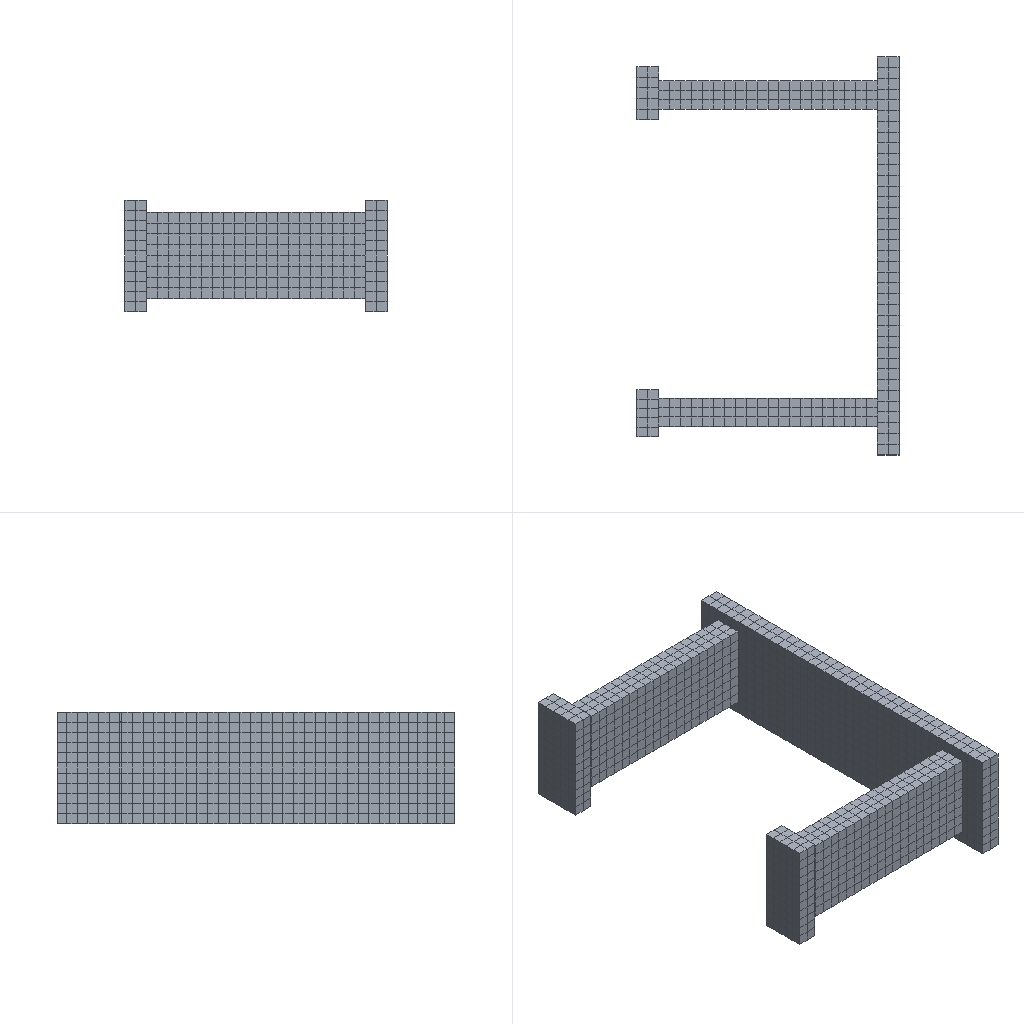Simulation study | ansys workbench
Set-up summary:
category,name,step,type,value,unit,region
solver,ansys_mapdl
solver,version,,,24.2
units,MPA,,stated
analysis,deck,,static,static
load_step,requested,,,1
analysis,nlgeom,,,False
mesh,nodes,,,11772
mesh,elements,,,2933
element_type,ANSYS 186 (type 1),,solid,110
element_type,ANSYS 186 (type 2),,solid,110
element_type,ANSYS 186 (type 3),,solid,480
element_type,ANSYS 186 (type 4),,solid,480
element_type,ANSYS 186 (type 5),,solid,814
element_type,ANSYS 174 (type 6),,contact,64
element_type,ANSYS 170 (type 7),,target,64
element_type,ANSYS 174 (type 8),,contact,74
element_type,ANSYS 170 (type 9),,target,74
element_type,ANSYS 174 (type 10),,contact,64
element_type,ANSYS 170 (type 11),,target,64
element_type,ANSYS 174 (type 12),,contact,64
element_type,ANSYS 170 (type 13),,target,64
element_type,ANSYS 154 (type 14),,surface,407
load,load commands in deck,,count,4
bc,support commands in deck,,count,1
named_set,_FIXEDSU,,component
material,1,,in results
material,2,,in results
material,3,,in results
material,4,,in results
material,5,,in results
check,setup vs results,,match,266 contact/target element(s) of the setup are not in the results: jiaoxue/qq_files/dp0/SYS/MECH/solve.out records that the solver deleted 266 by its trimming logic; 407 surface effect element(s) are not in the reader's mesh and were not compared
Ansys APDL input file, long lists of numbers shortened:
/batch
/config,noeldb,1     ! force off writing results to database
*get,_wallstrt,active,,time,wall
! ANSYS input file written by Workbench version 2024 R2
! File used for geometry attach: F:\jiaoxue\qq_files\dp0\SYS\DM\SYS.scdoc
/title,qq--____ (A5)
! ****** Begin Custom Load Command Snippet ******
/COM, ACT Extensions:
/COM,     LSDYNA, 2024.2
/COM,/COM,     ANSYSMotion, 2024.2
/COM,
! ****** End   Custom Load Command Snippet ******
*DIM,_wb_ProjectScratch_dir,string,248
_wb_ProjectScratch_dir(1) = 'F:\jiaoxue\_ProjectScratch\Scr3192\'
*DIM,_wb_SolverFiles_dir,string,248
_wb_SolverFiles_dir(1) = 'F:\jiaoxue\qq_files\dp0\SYS\MECH\'
*DIM,_wb_userfiles_dir,string,248
_wb_userfiles_dir(1) = 'F:\jiaoxue\qq_files\user_files\'
/com,--- Data in consistent NMM units. See Solving Units in the help system for more information.
/units,MPA
/nopr
/wb,file,start              !  signify a WB generated input file
/prep7
! Turn off shape checking because checks already performed inside WB mesher.
! See help system for more information.
SHPP,OFF,,NOWARN
/nolist
etcon,set             ! allow ANSYS to choose best KEYOP's for 180x elements, resets any applicable keyopt to MAPDL defaults
/com,*********** Nodes for the whole assembly ***********
nblock,3,,12949
(1i9,3e20.9e3)
        1    -1.050000000E+02     1.581539813E+02    -4.636363636E+01
! (11771 more lines like these left out)
-1
/wb,elem,start            !  set before creation of elements
/com,*********** Elements for Body 1 '1-prt0\__1' ***********
et,1,186
keyo,1,2,1          ! set full integration on SOLID186
eblock,19,solid,,110
(19i9)
        1        1        1        1        0        0        0        0       20        0        1        1      165      173      197       80      169      174      216
! (219 more lines like these left out)
-1
/com,*********** Elements for Body 2 '1-prt1\__1' ***********
et,2,186
keyo,2,2,1          ! set full integration on SOLID186
eblock,19,solid,,110
(19i9)
        2        2        2        2        0        0        0        0       20        0      111      739      915      936      950      818      934      935      951
! (219 more lines like these left out)
-1
/com,*********** Elements for Body 3 '1-prt2\__1' ***********
et,3,186
keyo,3,2,1          ! set full integration on SOLID186
eblock,19,solid,,480
(19i9)
        3        3        3        3        0        0        0        0       20        0      221     1477     2092     2117     2119     1875     2106     2116     2175
! (959 more lines like these left out)
-1
/com,*********** Elements for Body 4 '1-prt3\__1' ***********
et,4,186
keyo,4,2,1          ! set full integration on SOLID186
eblock,19,solid,,480
(19i9)
        4        4        4        4        0        0        0        0       20        0      701     4192     4906     4841     4817     4590     4920     4840     4836
! (959 more lines like these left out)
-1
/com,*********** Elements for Body 5 '1-prt4\__1' ***********
et,5,186
keyo,5,2,1          ! set full integration on SOLID186
eblock,19,solid,,814
(19i9)
        5        5        5        5        0        0        0        0       20        0     1181     6907     8107     8128     8203     7626     8126     8127     8239
! (1627 more lines like these left out)
-1
/wb,elem,end               !  done creating elements
/com,*********** Send User Defined Coordinate System(s) ***********
csys,0
toffst,273.15,      ! Temperature offset from absolute zero
/com,*********** Set Reference Temperature ***********
tref,22.
/wb,mat,start              !  starting to send materials
/com,*********** Send Materials ***********
Temperature = 'TEMP' ! Temperature
MP,DENS,1,7.85e-09,	! tonne mm^-3
MP,ALPX,1,1.2e-05,	! C^-1
MP,C,1,434000000,	! mm^2 s^-2 C^-1
MP,KXX,1,60.5,	! tonne mm s^-3 C^-1
MP,RSVX,1,0.00017,	! ohm mm
MP,EX,1,200000,	! tonne s^-2 mm^-1
MP,NUXY,1,0.3,
MP,MURX,1,10000,
Temperature = 'TEMP' ! Temperature
MP,DENS,2,7.85e-09,	! tonne mm^-3
MP,ALPX,2,1.2e-05,	! C^-1
MP,C,2,434000000,	! mm^2 s^-2 C^-1
MP,KXX,2,60.5,	! tonne mm s^-3 C^-1
MP,RSVX,2,0.00017,	! ohm mm
MP,EX,2,200000,	! tonne s^-2 mm^-1
MP,NUXY,2,0.3,
MP,MURX,2,10000,
Temperature = 'TEMP' ! Temperature
MP,DENS,3,7.85e-09,	! tonne mm^-3
MP,ALPX,3,1.2e-05,	! C^-1
MP,C,3,434000000,	! mm^2 s^-2 C^-1
MP,KXX,3,60.5,	! tonne mm s^-3 C^-1
MP,RSVX,3,0.00017,	! ohm mm
MP,EX,3,200000,	! tonne s^-2 mm^-1
MP,NUXY,3,0.3,
MP,MURX,3,10000,
Temperature = 'TEMP' ! Temperature
MP,DENS,4,7.85e-09,	! tonne mm^-3
MP,ALPX,4,1.2e-05,	! C^-1
MP,C,4,434000000,	! mm^2 s^-2 C^-1
MP,KXX,4,60.5,	! tonne mm s^-3 C^-1
MP,RSVX,4,0.00017,	! ohm mm
MP,EX,4,200000,	! tonne s^-2 mm^-1
MP,NUXY,4,0.3,
MP,MURX,4,10000,
Temperature = 'TEMP' ! Temperature
MP,DENS,5,7.85e-09,	! tonne mm^-3
MP,ALPX,5,1.2e-05,	! C^-1
MP,C,5,434000000,	! mm^2 s^-2 C^-1
MP,KXX,5,60.5,	! tonne mm s^-3 C^-1
MP,RSVX,5,0.00017,	! ohm mm
MP,EX,5,200000,	! tonne s^-2 mm^-1
MP,NUXY,5,0.3,
MP,MURX,5,10000,
/wb,mat,end                !  done sending materials
!************************* Model Summary ********************
!1-prt0\åºä½1,	ç»æé¢,	matid,	1
!1-prt1\åºä½1,	ç»æé¢,	matid,	2
!1-prt2\åºä½1,	ç»æé¢,	matid,	3
!1-prt3\åºä½1,	ç»æé¢,	matid,	4
!1-prt4\åºä½1,	ç»æé¢,	matid,	5
!************************* End Model Summary ********************
! get the diagonal of the bounding box. Needed later for other things
*get,_xmin,node,,mnloc,x
*get,_ymin,node,,mnloc,y
*get,_zmin,node,,mnloc,z
*get,_xmax,node,,mxloc,x
*get,_ymax,node,,mxloc,y
*get,_zmax,node,,mxloc,z
_ASMDIAG=(_xmax-_xmin)*(_xmax-_xmin)+(_ymax-_ymin)*(_ymax-_ymin)+(_zmax-_zmin)*(_zmax-_zmin)
_ASMDIAG=SQRT(_ASMDIAG)
/wb,contact,start          !  starting to send contact
/com,*********** Create Contact "½Ó´¥ÇøÓò" ***********
/com,            Real Constant Set For Above Contact Is 7 & 6
*set,tid,7
*set,cid,6
r,tid
r,cid
et,tid,170
et,cid,174
eblock,10,,,40
(15i9)
     4325        7        7        7        0       81       82      122      121      485      491      579      487
! (39 more lines like these left out)
-1
eblock,10,,,40
(15i9)
     4365        6        6        6        0       81       82      122      121      485      491      579      487
! (39 more lines like these left out)
-1
eblock,10,,,24
(15i9)
     4405        6        7        6        0     2057     2065     2091     2056     3898     3914     3896     3895
! (23 more lines like these left out)
-1
eblock,10,,,24
(15i9)
     4429        7        6        7        0     2057     2065     2091     2056     3898     3914     3896     3895
! (23 more lines like these left out)
-1
keyo,cid,8,2               ! auto create asymmetric contact (from Program Controlled setting)
keyo,cid,10,0              ! adjust contact stiffness each NR iteration (from Program Controlled setting)
keyo,cid,12,5              ! bonded always
keyo,cid,18,1              ! small sliding turned on by application
keyo,cid,2,2               ! MPC for bonded contacts (from Program Controlled setting)
keyo,tid,5,0               ! Automatic constraint type detection
keyo,cid,4,2               ! on nodal point - normal to target surface (from Program Controlled setting)
keyo,cid,9,1               ! ignore initial gaps/penetration
keyo,cid,7,0               ! No Prediction
rmod,tid,3,10.      ! FKN
rmod,tid,5,0.       ! ICONT
rmod,tid,6,0.       ! PINB
rmod,tid,10,0.      ! CNOF
rmod,tid,12,0.      ! FKT
rmod,tid,36,39      ! WB DSID
rmod,cid,3,10.      ! FKN
rmod,cid,5,0.       ! ICONT
rmod,cid,6,0.       ! PINB
rmod,cid,10,0.      ! CNOF
rmod,cid,12,0.      ! FKT
rmod,cid,36,39      ! WB DSID
/com,*********** Create Contact "½Ó´¥ÇøÓò 2" ***********
/com,            Real Constant Set For Above Contact Is 9 & 8
*set,tid,9
*set,cid,8
r,tid
r,cid
et,tid,170
et,cid,174
eblock,10,,,50
(15i9)
     4453        9        9        9        0      818      814      933      934     1212     1213     1449     1221
! (49 more lines like these left out)
-1
eblock,10,,,50
(15i9)
     4503        8        8        8        0      818      814      933      934     1212     1213     1449     1221
! (49 more lines like these left out)
-1
eblock,10,,,24
(15i9)
     4553        8        9        8        0     4724     4927     4839     4779     6517     6729     6626     6516
! (23 more lines like these left out)
-1
eblock,10,,,24
(15i9)
     4577        9        8        9        0     4724     4927     4839     4779     6517     6729     6626     6516
! (23 more lines like these left out)
-1
keyo,cid,8,2               ! auto create asymmetric contact (from Program Controlled setting)
keyo,cid,10,0              ! adjust contact stiffness each NR iteration (from Program Controlled setting)
keyo,cid,12,5              ! bonded always
keyo,cid,18,1              ! small sliding turned on by application
keyo,cid,2,2               ! MPC for bonded contacts (from Program Controlled setting)
keyo,tid,5,0               ! Automatic constraint type detection
keyo,cid,4,2               ! on nodal point - normal to target surface (from Program Controlled setting)
keyo,cid,9,1               ! ignore initial gaps/penetration
keyo,cid,7,0               ! No Prediction
rmod,tid,3,10.      ! FKN
rmod,tid,5,0.       ! ICONT
rmod,tid,6,0.       ! PINB
rmod,tid,10,0.      ! CNOF
rmod,tid,12,0.      ! FKT
rmod,tid,36,42      ! WB DSID
rmod,cid,3,10.      ! FKN
rmod,cid,5,0.       ! ICONT
rmod,cid,6,0.       ! PINB
rmod,cid,10,0.      ! CNOF
rmod,cid,12,0.      ! FKT
rmod,cid,36,42      ! WB DSID
/com,*********** Create Contact "½Ó´¥ÇøÓò 3" ***********
/com,            Real Constant Set For Above Contact Is 11 & 10
*set,tid,11
*set,cid,10
r,tid
r,cid
et,tid,170
et,cid,174
eblock,10,,,24
(15i9)
     4601       11       11       11        0     2106     2092     2117     2116     3962     3963     4003     3991
! (23 more lines like these left out)
-1
eblock,10,,,24
(15i9)
     4625       10       10       10        0     2106     2092     2117     2116     3962     3963     4003     3991
! (23 more lines like these left out)
-1
eblock,10,,,40
(15i9)
     4649       10       11       10        0     8270     7595     7596     8269    10464    10463    10466    11768
! (39 more lines like these left out)
-1
eblock,10,,,40
(15i9)
     4689       11       10       11        0     8270     7595     7596     8269    10464    10463    10466    11768
! (39 more lines like these left out)
-1
keyo,cid,8,2               ! auto create asymmetric contact (from Program Controlled setting)
keyo,cid,10,0              ! adjust contact stiffness each NR iteration (from Program Controlled setting)
keyo,cid,12,5              ! bonded always
keyo,cid,18,1              ! small sliding turned on by application
keyo,cid,2,2               ! MPC for bonded contacts (from Program Controlled setting)
keyo,tid,5,0               ! Automatic constraint type detection
keyo,cid,4,2               ! on nodal point - normal to target surface (from Program Controlled setting)
keyo,cid,9,1               ! ignore initial gaps/penetration
keyo,cid,7,0               ! No Prediction
rmod,tid,3,10.      ! FKN
rmod,tid,5,0.       ! ICONT
rmod,tid,6,0.       ! PINB
rmod,tid,10,0.      ! CNOF
rmod,tid,12,0.      ! FKT
rmod,tid,36,45      ! WB DSID
rmod,cid,3,10.      ! FKN
rmod,cid,5,0.       ! ICONT
rmod,cid,6,0.       ! PINB
rmod,cid,10,0.      ! CNOF
rmod,cid,12,0.      ! FKT
rmod,cid,36,45      ! WB DSID
/com,*********** Create Contact "½Ó´¥ÇøÓò 4" ***********
/com,            Real Constant Set For Above Contact Is 13 & 12
*set,tid,13
*set,cid,12
r,tid
r,cid
et,tid,170
et,cid,174
eblock,10,,,24
(15i9)
     4729       13       13       13        0     4920     4906     4841     4840     6845     6733     6730     6731
! (23 more lines like these left out)
-1
eblock,10,,,24
(15i9)
     4753       12       12       12        0     4920     4906     4841     4840     6845     6733     6730     6731
! (23 more lines like these left out)
-1
eblock,10,,,40
(15i9)
     4777       12       13       12        0     8241     7624     7625     8240    10522    10521    10524    11739
! (39 more lines like these left out)
-1
eblock,10,,,40
(15i9)
     4817       13       12       13        0     8241     7624     7625     8240    10522    10521    10524    11739
! (39 more lines like these left out)
-1
keyo,cid,8,2               ! auto create asymmetric contact (from Program Controlled setting)
keyo,cid,10,0              ! adjust contact stiffness each NR iteration (from Program Controlled setting)
keyo,cid,12,5              ! bonded always
keyo,cid,18,1              ! small sliding turned on by application
keyo,cid,2,2               ! MPC for bonded contacts (from Program Controlled setting)
keyo,tid,5,0               ! Automatic constraint type detection
keyo,cid,4,2               ! on nodal point - normal to target surface (from Program Controlled setting)
keyo,cid,9,1               ! ignore initial gaps/penetration
keyo,cid,7,0               ! No Prediction
rmod,tid,3,10.      ! FKN
rmod,tid,5,0.       ! ICONT
rmod,tid,6,0.       ! PINB
rmod,tid,10,0.      ! CNOF
rmod,tid,12,0.      ! FKT
rmod,tid,36,48      ! WB DSID
rmod,cid,3,10.      ! FKN
rmod,cid,5,0.       ! ICONT
rmod,cid,6,0.       ! PINB
rmod,cid,10,0.      ! CNOF
rmod,cid,12,0.      ! FKT
rmod,cid,36,48      ! WB DSID
nsel,all
esel,all
/wb,contact,end            !  done creating contacts
/golist
/wb,load,start             !  starting to send loads
/com,*********** Fixed Supports ***********
CMBLOCK,_FIXEDSU,NODE,      396
(8i10)
        41        42        43        44        45        46        47        48
! (49 more lines like these left out)
cmsel,s,_FIXEDSU
d,all,all
nsel,all
/com,*********** Define Force Using Surface Effect Elements ***********
local,12,0,0.,0.,0.,0.,0.,0.
csys,0
et,14,154
mat,14
eblock,10,,,407
(15i9)
     4857       14       14       14       12     8060     7627     8022     8059    10530    10529    11364    11439
! (406 more lines like these left out)
-1
esel,s,type,,14
keyop,14,2,1        ! Apply load in local coordinate system
keyop,14,7,1        ! Use original area so load is constant in large deformation
esel,all
/gst,on,on
fini
*get,_numnode,node,0,count
*get,_numelem,elem,0,count
*get, _MAXELEMNUM, elem, 0, NUM, MAX
*get, _MAXNODENUM, node, 0, NUM, MAX
*get, _MAXELEMTYPE, etyp, 0, NUM, MAX
*get, _MAXREALCONST, rcon, 0, NUM, MAX
/go
/wb,load,end               !  done creating loads
/com,--- Number of total nodes = %_numnode%
/com,--- Number of contact elements = 939
/com,--- Number of spring elements = 0
/com,--- Number of bearing elements = 0
/com,--- Number of solid elements = 1994
/com,--- Number of condensed parts = 0
/com,--- Number of total elements = %_numelem%
*get,_wallbsol,active,,time,wall
/com,****************************************************************************
/com,*************************    SOLUTION       ********************************
/com,****************************************************************************
/solu
antype,0                   ! static analysis
_thickRatio=0.4     ! Ratio of thick parts in the model
eqsl,sparse,,,,,1
cntr,print,1               ! print out contact info and also make no initial contact an error
cncheck,dmp		!	Enable program controlled contact splitting for distributed memory parallel run
dmpoption,emat,no             ! Don't combine emat file for DANSYS
dmpoption,esav,no             ! Don't combine esav file for DANSYS
nldiag,cont,iter           ! print out contact info each equilibrium iteration
rescontrol,,none                 ! Do not keep any restart files
/com,****************************************************
/com,******************* SOLVE FOR LS 1 OF 1 ****************
esel,s,type,,14
nsle
sfe,all,1,pres,1,-0.1077
sfe,all,2,pres,1,0.
sfe,all,3,pres,1,0.
nsel,all
esel,all
acel,9806.65,0.,0.
/nopr
/gopr
nsub,1,1,1
time,1.
outres,erase
outres,all,none
outres,nsol,all,
outres,rsol,all
outres,eangl,all
outres,etmp,all
outres,veng,all
outres,strs,all,
outres,epel,all,
outres,eppl,all,
outres,cont,all,
! *********** WB SOLVE COMMAND ***********
! check interactive state
*get,ANSINTER_,active,,int
*if,ANSINTER_,ne,0,then
/eof
*endif
solve
/com *************** Write FE CONNECTORS *********
CEWRITE,file,ce,,INTE
/com,****************************************************
/com,*************** FINISHED SOLVE FOR LS 1 *************
*get,_wallasol,active,,time,wall
/nopr
*get,_numnode,node,0,count
*get,_numelem,elem,0,count
*get, _MAXELEMNUM, elem, 0, NUM, MAX
*get, _MAXNODENUM, node, 0, NUM, MAX,,,INTERNAL
*get, _MAXELEMTYPE, etyp, 0, NUM, MAX
*get, _MAXREALCONST, rcon, 0, NUM, MAX
*get,_NSOLTHREADS,active,0,ntfs
*get,_NSOLPROCESSES,active,0,npfs
/gopr
/post1
xmlo,ENCODING,ISO-8859-1
xmlo,parm
/xml,parm,xml
fini
/gopr
*get,_walldone,active,,time,wall
_preptime=(_wallbsol-_wallstrt)*3600
_solvtime=(_wallasol-_wallbsol)*3600
_posttime=(_walldone-_wallasol)*3600
_totaltim=(_walldone-_wallstrt)*3600
*get,_dlbratio,active,0,solu,dlbr
*get,_combtime,active,0,solu,comb
*get,_ssmode,active,0,solu,ssmm
*get,_ndofs,active,0,solu,ndof
*get,_sol_end_time,active,0,set,time
*if,_sol_end_time,eq,1.,then
/fclean				!clean distributed files
*endif
/com,--- Total number of nodes = %_numnode%
/com,--- Total number of elements = %_numelem%
/com,--- Element load balance ratio = %_dlbratio%
/com,--- Time to combine distributed files = %_combtime%
/com,--- Sparse memory mode = %_ssmode%
/com,--- Number of DOF = %_ndofs%
/wb,file,end               ! done with WB generated input
Results summary:
result,analysis,,,static
result,last_loadstep,,,1
result,primary field,,,displacement
result,reaction total,1,FX,1016.821,N
result,reaction total,1,FY,-0.0,N
result,reaction total,1,FZ,0.0,N
result,mass,,,0.001715,"NMM: mm, ton, N, s, mV, mA, degC"